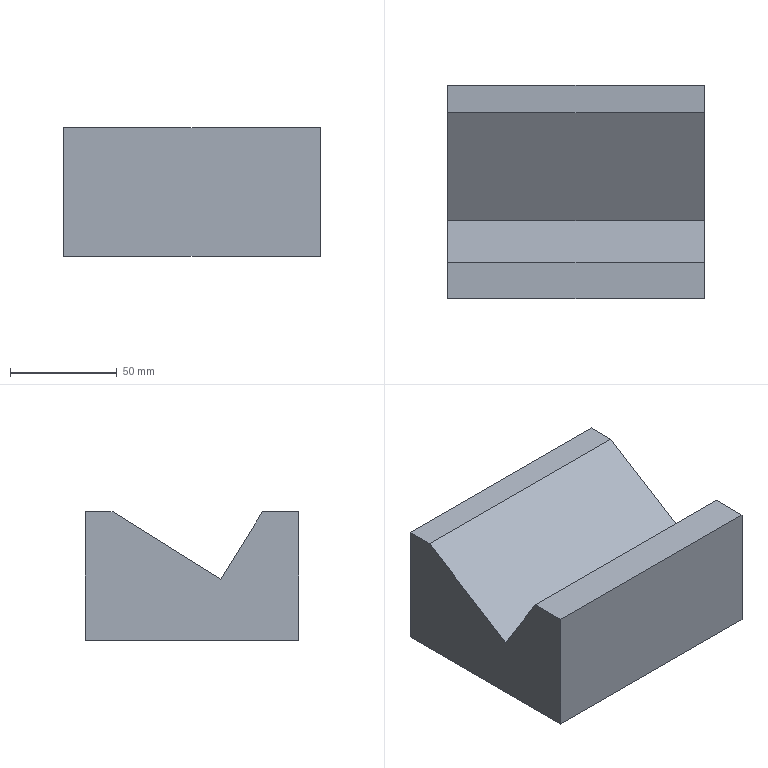Part | Mastercam | 1 solid | 9 faces | box 120 x 100 x 60 mm | volume 587811 mm3 | plane 9
STEP:
#1=CARTESIAN_POINT('',(0.,0.,0.));
#2=DIRECTION('',(0.,0.,1.));
#3=DIRECTION('',(1.,0.,0.));
#4=AXIS2_PLACEMENT_3D('',#1,#2,#3);
#5=CARTESIAN_POINT('',(-60.,46.414,-5.));
#6=VERTEX_POINT('',#5);
#7=CARTESIAN_POINT('',(60.,46.414,-5.));
#8=VERTEX_POINT('',#7);
#9=CARTESIAN_POINT('',(-60.,46.414,-5.));
#10=DIRECTION('',(1.,0.,0.));
#11=VECTOR('',#10,1.);
#12=LINE('',#9,#11);
#13=EDGE_CURVE('',#6,#8,#12,.T.);
#14=ORIENTED_EDGE('',*,*,#13,.T.);
#15=CARTESIAN_POINT('',(60.,46.414,-65.));
#16=VERTEX_POINT('',#15);
#17=CARTESIAN_POINT('',(60.,46.414,-5.));
#18=DIRECTION('',(0.,0.,-1.));
#19=VECTOR('',#18,1.);
#20=LINE('',#17,#19);
#21=EDGE_CURVE('',#8,#16,#20,.T.);
#22=ORIENTED_EDGE('',*,*,#21,.T.);
#23=CARTESIAN_POINT('',(-60.,46.414,-65.));
#24=VERTEX_POINT('',#23);
#25=CARTESIAN_POINT('',(-60.,46.414,-65.));
#26=DIRECTION('',(1.,0.,0.));
#27=VECTOR('',#26,1.);
#28=LINE('',#25,#27);
#29=EDGE_CURVE('',#24,#16,#28,.T.);
#30=ORIENTED_EDGE('',*,*,#29,.F.);
#31=CARTESIAN_POINT('',(-60.,46.414,-5.));
#32=DIRECTION('',(0.,0.,-1.));
#33=VECTOR('',#32,1.);
#34=LINE('',#31,#33);
#35=EDGE_CURVE('',#6,#24,#34,.T.);
#36=ORIENTED_EDGE('',*,*,#35,.F.);
#37=EDGE_LOOP('',(#14,#22,#30,#36));
#38=FACE_OUTER_BOUND('',#37,.T.);
#39=CARTESIAN_POINT('',(-60.,46.414,-5.));
#40=DIRECTION('',(0.,-1.,0.));
#41=DIRECTION('',(0.,0.,1.));
#42=AXIS2_PLACEMENT_3D('',#39,#40,#41);
#43=PLANE('',#42);
#44=ADVANCED_FACE('',(#38),#43,.F.);
#45=ORIENTED_EDGE('',*,*,#29,.T.);
#46=CARTESIAN_POINT('',(60.,-53.587,-65.));
#47=VERTEX_POINT('',#46);
#48=CARTESIAN_POINT('',(60.,41.414,-65.));
#49=DIRECTION('',(0.,-1.,0.));
#50=VECTOR('',#49,1.);
#51=LINE('',#48,#50);
#52=EDGE_CURVE('',#16,#47,#51,.T.);
#53=ORIENTED_EDGE('',*,*,#52,.T.);
#54=CARTESIAN_POINT('',(-60.,-53.587,-65.));
#55=VERTEX_POINT('',#54);
#56=CARTESIAN_POINT('',(-60.,-53.587,-65.));
#57=DIRECTION('',(1.,0.,0.));
#58=VECTOR('',#57,1.);
#59=LINE('',#56,#58);
#60=EDGE_CURVE('',#55,#47,#59,.T.);
#61=ORIENTED_EDGE('',*,*,#60,.F.);
#62=CARTESIAN_POINT('',(-60.,41.414,-65.));
#63=DIRECTION('',(0.,-1.,0.));
#64=VECTOR('',#63,1.);
#65=LINE('',#62,#64);
#66=EDGE_CURVE('',#24,#55,#65,.T.);
#67=ORIENTED_EDGE('',*,*,#66,.F.);
#68=EDGE_LOOP('',(#45,#53,#61,#67));
#69=FACE_OUTER_BOUND('',#68,.T.);
#70=CARTESIAN_POINT('',(-60.,41.414,-65.));
#71=DIRECTION('',(0.,0.,1.));
#72=DIRECTION('',(-1.,0.,0.));
#73=AXIS2_PLACEMENT_3D('',#70,#71,#72);
#74=PLANE('',#73);
#75=ADVANCED_FACE('',(#69),#74,.F.);
#76=ORIENTED_EDGE('',*,*,#60,.T.);
#77=CARTESIAN_POINT('',(60.,-53.587,-5.));
#78=VERTEX_POINT('',#77);
#79=CARTESIAN_POINT('',(60.,-53.587,-5.));
#80=DIRECTION('',(0.,0.,-1.));
#81=VECTOR('',#80,1.);
#82=LINE('',#79,#81);
#83=EDGE_CURVE('',#78,#47,#82,.T.);
#84=ORIENTED_EDGE('',*,*,#83,.F.);
#85=CARTESIAN_POINT('',(-60.,-53.587,-5.));
#86=VERTEX_POINT('',#85);
#87=CARTESIAN_POINT('',(-60.,-53.587,-5.));
#88=DIRECTION('',(1.,0.,0.));
#89=VECTOR('',#88,1.);
#90=LINE('',#87,#89);
#91=EDGE_CURVE('',#86,#78,#90,.T.);
#92=ORIENTED_EDGE('',*,*,#91,.F.);
#93=CARTESIAN_POINT('',(-60.,-53.587,-5.));
#94=DIRECTION('',(0.,0.,-1.));
#95=VECTOR('',#94,1.);
#96=LINE('',#93,#95);
#97=EDGE_CURVE('',#86,#55,#96,.T.);
#98=ORIENTED_EDGE('',*,*,#97,.T.);
#99=EDGE_LOOP('',(#76,#84,#92,#98));
#100=FACE_OUTER_BOUND('',#99,.T.);
#101=CARTESIAN_POINT('',(-60.,-53.587,-5.));
#102=DIRECTION('',(0.,-1.,0.));
#103=DIRECTION('',(0.,0.,1.));
#104=AXIS2_PLACEMENT_3D('',#101,#102,#103);
#105=PLANE('',#104);
#106=ADVANCED_FACE('',(#100),#105,.T.);
#107=ORIENTED_EDGE('',*,*,#91,.T.);
#108=CARTESIAN_POINT('',(60.,-36.606,-5.));
#109=VERTEX_POINT('',#108);
#110=CARTESIAN_POINT('',(60.,-39.731,-5.));
#111=DIRECTION('',(0.,1.,0.));
#112=VECTOR('',#111,1.);
#113=LINE('',#110,#112);
#114=EDGE_CURVE('',#78,#109,#113,.T.);
#115=ORIENTED_EDGE('',*,*,#114,.T.);
#116=CARTESIAN_POINT('',(-60.,-36.606,-5.));
#117=VERTEX_POINT('',#116);
#118=CARTESIAN_POINT('',(-60.,-36.606,-5.));
#119=DIRECTION('',(1.,0.,0.));
#120=VECTOR('',#119,1.);
#121=LINE('',#118,#120);
#122=EDGE_CURVE('',#117,#109,#121,.T.);
#123=ORIENTED_EDGE('',*,*,#122,.F.);
#124=CARTESIAN_POINT('',(-60.,-39.731,-5.));
#125=DIRECTION('',(0.,1.,0.));
#126=VECTOR('',#125,1.);
#127=LINE('',#124,#126);
#128=EDGE_CURVE('',#86,#117,#127,.T.);
#129=ORIENTED_EDGE('',*,*,#128,.F.);
#130=EDGE_LOOP('',(#107,#115,#123,#129));
#131=FACE_OUTER_BOUND('',#130,.T.);
#132=CARTESIAN_POINT('',(-60.,-39.731,-5.));
#133=DIRECTION('',(0.,0.,-1.));
#134=DIRECTION('',(0.,-1.,0.));
#135=AXIS2_PLACEMENT_3D('',#132,#133,#134);
#136=PLANE('',#135);
#137=ADVANCED_FACE('',(#131),#136,.F.);
#138=ORIENTED_EDGE('',*,*,#122,.T.);
#139=CARTESIAN_POINT('',(60.,-16.944,-36.466));
#140=VERTEX_POINT('',#139);
#141=CARTESIAN_POINT('',(60.,-36.606,-5.));
#142=DIRECTION('',(0.,0.5299,-0.848));
#143=VECTOR('',#142,1.);
#144=LINE('',#141,#143);
#145=EDGE_CURVE('',#109,#140,#144,.T.);
#146=ORIENTED_EDGE('',*,*,#145,.T.);
#147=CARTESIAN_POINT('',(-60.,-16.944,-36.466));
#148=VERTEX_POINT('',#147);
#149=CARTESIAN_POINT('',(-60.,-16.944,-36.466));
#150=DIRECTION('',(1.,0.,0.));
#151=VECTOR('',#150,1.);
#152=LINE('',#149,#151);
#153=EDGE_CURVE('',#148,#140,#152,.T.);
#154=ORIENTED_EDGE('',*,*,#153,.F.);
#155=CARTESIAN_POINT('',(-60.,-36.606,-5.));
#156=DIRECTION('',(0.,0.5299,-0.848));
#157=VECTOR('',#156,1.);
#158=LINE('',#155,#157);
#159=EDGE_CURVE('',#117,#148,#158,.T.);
#160=ORIENTED_EDGE('',*,*,#159,.F.);
#161=EDGE_LOOP('',(#138,#146,#154,#160));
#162=FACE_OUTER_BOUND('',#161,.T.);
#163=CARTESIAN_POINT('',(-60.,-36.606,-5.));
#164=DIRECTION('',(0.,-0.848,-0.5299));
#165=DIRECTION('',(0.,-0.5299,0.848));
#166=AXIS2_PLACEMENT_3D('',#163,#164,#165);
#167=PLANE('',#166);
#168=ADVANCED_FACE('',(#162),#167,.F.);
#169=CARTESIAN_POINT('',(-60.,33.412,-5.));
#170=VERTEX_POINT('',#169);
#171=CARTESIAN_POINT('',(-60.,33.412,-5.));
#172=DIRECTION('',(0.,-0.848,-0.5299));
#173=VECTOR('',#172,1.);
#174=LINE('',#171,#173);
#175=EDGE_CURVE('',#170,#148,#174,.T.);
#176=ORIENTED_EDGE('',*,*,#175,.T.);
#177=ORIENTED_EDGE('',*,*,#153,.T.);
#178=CARTESIAN_POINT('',(60.,33.412,-5.));
#179=VERTEX_POINT('',#178);
#180=CARTESIAN_POINT('',(60.,33.412,-5.));
#181=DIRECTION('',(0.,-0.848,-0.5299));
#182=VECTOR('',#181,1.);
#183=LINE('',#180,#182);
#184=EDGE_CURVE('',#179,#140,#183,.T.);
#185=ORIENTED_EDGE('',*,*,#184,.F.);
#186=CARTESIAN_POINT('',(-60.,33.412,-5.));
#187=DIRECTION('',(1.,0.,0.));
#188=VECTOR('',#187,1.);
#189=LINE('',#186,#188);
#190=EDGE_CURVE('',#170,#179,#189,.T.);
#191=ORIENTED_EDGE('',*,*,#190,.F.);
#192=EDGE_LOOP('',(#176,#177,#185,#191));
#193=FACE_OUTER_BOUND('',#192,.T.);
#194=CARTESIAN_POINT('',(-60.,33.412,-5.));
#195=DIRECTION('',(0.,-0.5299,0.848));
#196=DIRECTION('',(0.,0.848,0.5299));
#197=AXIS2_PLACEMENT_3D('',#194,#195,#196);
#198=PLANE('',#197);
#199=ADVANCED_FACE('',(#193),#198,.T.);
#200=ORIENTED_EDGE('',*,*,#190,.T.);
#201=CARTESIAN_POINT('',(60.,41.414,-5.));
#202=DIRECTION('',(0.,-1.,0.));
#203=VECTOR('',#202,1.);
#204=LINE('',#201,#203);
#205=EDGE_CURVE('',#8,#179,#204,.T.);
#206=ORIENTED_EDGE('',*,*,#205,.F.);
#207=ORIENTED_EDGE('',*,*,#13,.F.);
#208=CARTESIAN_POINT('',(-60.,41.414,-5.));
#209=DIRECTION('',(0.,-1.,0.));
#210=VECTOR('',#209,1.);
#211=LINE('',#208,#210);
#212=EDGE_CURVE('',#6,#170,#211,.T.);
#213=ORIENTED_EDGE('',*,*,#212,.T.);
#214=EDGE_LOOP('',(#200,#206,#207,#213));
#215=FACE_OUTER_BOUND('',#214,.T.);
#216=CARTESIAN_POINT('',(-60.,41.414,-5.));
#217=DIRECTION('',(0.,0.,1.));
#218=DIRECTION('',(-1.,0.,0.));
#219=AXIS2_PLACEMENT_3D('',#216,#217,#218);
#220=PLANE('',#219);
#221=ADVANCED_FACE('',(#215),#220,.T.);
#222=ORIENTED_EDGE('',*,*,#159,.T.);
#223=ORIENTED_EDGE('',*,*,#175,.F.);
#224=ORIENTED_EDGE('',*,*,#212,.F.);
#225=ORIENTED_EDGE('',*,*,#35,.T.);
#226=ORIENTED_EDGE('',*,*,#66,.T.);
#227=ORIENTED_EDGE('',*,*,#97,.F.);
#228=ORIENTED_EDGE('',*,*,#128,.T.);
#229=EDGE_LOOP('',(#222,#223,#224,#225,#226,#227,#228));
#230=FACE_OUTER_BOUND('',#229,.T.);
#231=CARTESIAN_POINT('',(-60.,0.,0.));
#232=DIRECTION('',(-1.,0.,0.));
#233=DIRECTION('',(0.,0.,-1.));
#234=AXIS2_PLACEMENT_3D('',#231,#232,#233);
#235=PLANE('',#234);
#236=ADVANCED_FACE('',(#230),#235,.T.);
#237=ORIENTED_EDGE('',*,*,#184,.T.);
#238=ORIENTED_EDGE('',*,*,#145,.F.);
#239=ORIENTED_EDGE('',*,*,#114,.F.);
#240=ORIENTED_EDGE('',*,*,#83,.T.);
#241=ORIENTED_EDGE('',*,*,#52,.F.);
#242=ORIENTED_EDGE('',*,*,#21,.F.);
#243=ORIENTED_EDGE('',*,*,#205,.T.);
#244=EDGE_LOOP('',(#237,#238,#239,#240,#241,#242,#243));
#245=FACE_OUTER_BOUND('',#244,.T.);
#246=CARTESIAN_POINT('',(60.,0.,0.));
#247=DIRECTION('',(-1.,0.,0.));
#248=DIRECTION('',(0.,0.,-1.));
#249=AXIS2_PLACEMENT_3D('',#246,#247,#248);
#250=PLANE('',#249);
#251=ADVANCED_FACE('',(#245),#250,.F.);
#252=CLOSED_SHELL('',(#44,#75,#106,#137,#168,#199,#221,#236,#251));
#253=MANIFOLD_SOLID_BREP('',#252);
#254=(LENGTH_UNIT()NAMED_UNIT(*)SI_UNIT(.MILLI.,.METRE.));
#255=UNCERTAINTY_MEASURE_WITH_UNIT(LENGTH_MEASURE(0.005),#254,'','');
#256=(NAMED_UNIT(*)PLANE_ANGLE_UNIT()SI_UNIT($,.RADIAN.));
#257=(GEOMETRIC_REPRESENTATION_CONTEXT(3)GLOBAL_UNCERTAINTY_ASSIGNED_CONTEXT((#255))GLOBAL_UNIT_ASSIGNED_CONTEXT((#254,#256))REPRESENTATION_CONTEXT('',''));
#258=ADVANCED_BREP_SHAPE_REPRESENTATION('',(#4,#253),#257);